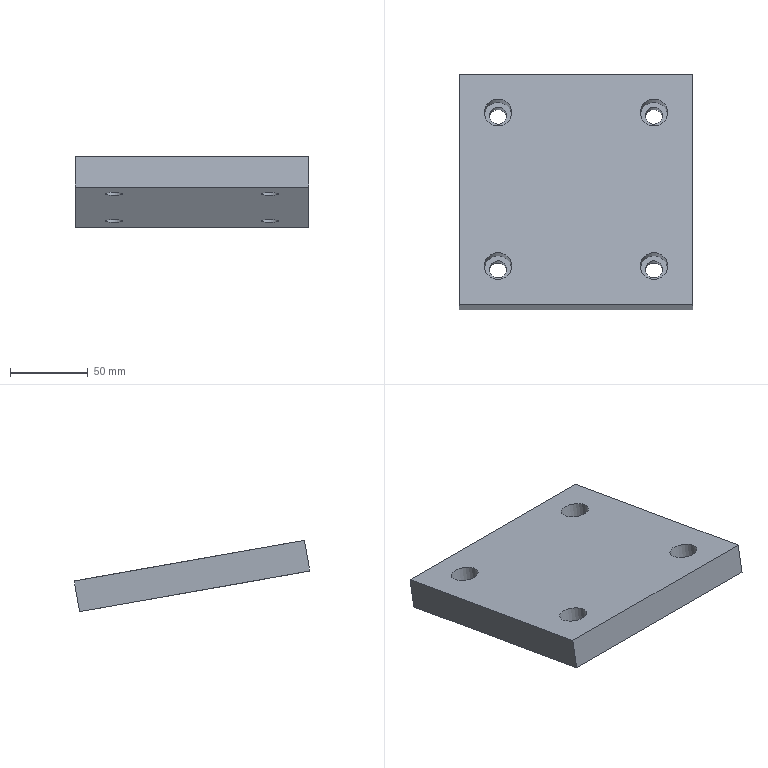Part | NX | features solid 2 | 1 solid | 18 faces | box 150 x 151.194 x 45.743 mm | volume 435414 mm3 | plane 10 | cylinder 8 | commonest cylinder face diameters 11 x4 17.5 x4
STEP:
#1=CARTESIAN_POINT('',(-801.6,-898.696,-239.036));
#2=VERTEX_POINT('',#1);
#3=CARTESIAN_POINT('',(-801.6,-902.169,-258.732));
#4=VERTEX_POINT('',#3);
#5=CARTESIAN_POINT('',(-801.6,-898.696,-239.036));
#6=DIRECTION('',(0.,0.1736,0.9848));
#7=VECTOR('',#6,1000.);
#8=LINE('',#5,#7);
#9=EDGE_CURVE('',#2,#4,#8,.F.);
#10=ORIENTED_EDGE('',*,*,#9,.T.);
#11=CARTESIAN_POINT('',(-951.6,-902.169,-258.732));
#12=VERTEX_POINT('',#11);
#13=CARTESIAN_POINT('',(-801.6,-902.169,-258.732));
#14=DIRECTION('',(1.,0.,0.));
#15=VECTOR('',#14,1000.);
#16=LINE('',#13,#15);
#17=EDGE_CURVE('',#4,#12,#16,.F.);
#18=ORIENTED_EDGE('',*,*,#17,.T.);
#19=CARTESIAN_POINT('',(-951.6,-898.696,-239.036));
#20=VERTEX_POINT('',#19);
#21=CARTESIAN_POINT('',(-951.6,-898.696,-239.036));
#22=DIRECTION('',(0.,-0.1736,-0.9848));
#23=VECTOR('',#22,1000.);
#24=LINE('',#21,#23);
#25=EDGE_CURVE('',#20,#12,#24,.T.);
#26=ORIENTED_EDGE('',*,*,#25,.F.);
#27=CARTESIAN_POINT('',(-801.6,-898.696,-239.036));
#28=DIRECTION('',(1.,0.,0.));
#29=VECTOR('',#28,1000.);
#30=LINE('',#27,#29);
#31=EDGE_CURVE('',#2,#20,#30,.F.);
#32=ORIENTED_EDGE('',*,*,#31,.F.);
#33=EDGE_LOOP('',(#10,#18,#26,#32));
#34=FACE_BOUND('',#33,.T.);
#35=CARTESIAN_POINT('',(-801.6,-898.696,-239.036));
#36=DIRECTION('',(0.,0.9848,-0.1736));
#37=DIRECTION('',(-1.,0.,0.));
#38=AXIS2_PLACEMENT_3D('',#35,#36,#37);
#39=PLANE('',#38);
#40=ADVANCED_FACE('',(#34),#39,.T.);
#41=ORIENTED_EDGE('',*,*,#25,.T.);
#42=CARTESIAN_POINT('',(-951.6,-1049.891,-232.685));
#43=VERTEX_POINT('',#42);
#44=CARTESIAN_POINT('',(-951.6,-852.929,-267.415));
#45=DIRECTION('',(0.,-0.9848,0.1736));
#46=VECTOR('',#45,1000.);
#47=LINE('',#44,#46);
#48=EDGE_CURVE('',#12,#43,#47,.T.);
#49=ORIENTED_EDGE('',*,*,#48,.T.);
#50=CARTESIAN_POINT('',(-951.6,-1046.418,-212.989));
#51=VERTEX_POINT('',#50);
#52=CARTESIAN_POINT('',(-951.6,-1046.418,-212.989));
#53=DIRECTION('',(0.,0.1736,0.9848));
#54=VECTOR('',#53,1000.);
#55=LINE('',#52,#54);
#56=EDGE_CURVE('',#51,#43,#55,.F.);
#57=ORIENTED_EDGE('',*,*,#56,.F.);
#58=CARTESIAN_POINT('',(-951.6,-849.456,-247.718));
#59=DIRECTION('',(0.,-0.9848,0.1736));
#60=VECTOR('',#59,1000.);
#61=LINE('',#58,#60);
#62=EDGE_CURVE('',#20,#51,#61,.T.);
#63=ORIENTED_EDGE('',*,*,#62,.F.);
#64=EDGE_LOOP('',(#41,#49,#57,#63));
#65=FACE_BOUND('',#64,.T.);
#66=CARTESIAN_POINT('',(-951.6,-849.456,-247.718));
#67=DIRECTION('',(-1.,0.,0.));
#68=DIRECTION('',(0.,-0.9848,0.1736));
#69=AXIS2_PLACEMENT_3D('',#66,#67,#68);
#70=PLANE('',#69);
#71=ADVANCED_FACE('',(#65),#70,.T.);
#72=ORIENTED_EDGE('',*,*,#56,.T.);
#73=CARTESIAN_POINT('',(-801.6,-1049.891,-232.685));
#74=VERTEX_POINT('',#73);
#75=CARTESIAN_POINT('',(-801.6,-1049.891,-232.685));
#76=DIRECTION('',(-1.,0.,0.));
#77=VECTOR('',#76,1000.);
#78=LINE('',#75,#77);
#79=EDGE_CURVE('',#74,#43,#78,.T.);
#80=ORIENTED_EDGE('',*,*,#79,.F.);
#81=CARTESIAN_POINT('',(-801.6,-1046.418,-212.989));
#82=VERTEX_POINT('',#81);
#83=CARTESIAN_POINT('',(-801.6,-1046.418,-212.989));
#84=DIRECTION('',(0.,0.1736,0.9848));
#85=VECTOR('',#84,1000.);
#86=LINE('',#83,#85);
#87=EDGE_CURVE('',#82,#74,#86,.F.);
#88=ORIENTED_EDGE('',*,*,#87,.F.);
#89=CARTESIAN_POINT('',(-801.6,-1046.418,-212.989));
#90=DIRECTION('',(-1.,0.,0.));
#91=VECTOR('',#90,1000.);
#92=LINE('',#89,#91);
#93=EDGE_CURVE('',#82,#51,#92,.T.);
#94=ORIENTED_EDGE('',*,*,#93,.T.);
#95=EDGE_LOOP('',(#72,#80,#88,#94));
#96=FACE_BOUND('',#95,.T.);
#97=CARTESIAN_POINT('',(-801.6,-1046.418,-212.989));
#98=DIRECTION('',(0.,0.9848,-0.1736));
#99=DIRECTION('',(-1.,0.,0.));
#100=AXIS2_PLACEMENT_3D('',#97,#98,#99);
#101=PLANE('',#100);
#102=ADVANCED_FACE('',(#96),#101,.F.);
#103=CARTESIAN_POINT('',(-801.6,-849.456,-247.718));
#104=DIRECTION('',(0.,-0.9848,0.1736));
#105=VECTOR('',#104,1000.);
#106=LINE('',#103,#105);
#107=EDGE_CURVE('',#2,#82,#106,.T.);
#108=ORIENTED_EDGE('',*,*,#107,.T.);
#109=ORIENTED_EDGE('',*,*,#87,.T.);
#110=CARTESIAN_POINT('',(-801.6,-852.929,-267.415));
#111=DIRECTION('',(0.,-0.9848,0.1736));
#112=VECTOR('',#111,1000.);
#113=LINE('',#110,#112);
#114=EDGE_CURVE('',#4,#74,#113,.T.);
#115=ORIENTED_EDGE('',*,*,#114,.F.);
#116=ORIENTED_EDGE('',*,*,#9,.F.);
#117=EDGE_LOOP('',(#108,#109,#115,#116));
#118=FACE_BOUND('',#117,.T.);
#119=CARTESIAN_POINT('',(-801.6,-849.456,-247.718));
#120=DIRECTION('',(-1.,0.,0.));
#121=DIRECTION('',(0.,-0.9848,0.1736));
#122=AXIS2_PLACEMENT_3D('',#119,#120,#121);
#123=PLANE('',#122);
#124=ADVANCED_FACE('',(#118),#123,.F.);
#125=CARTESIAN_POINT('',(-832.1,-926.79,-254.391));
#126=VERTEX_POINT('',#125);
#127=CARTESIAN_POINT('',(-826.6,-926.79,-254.391));
#128=DIRECTION('',(0.,0.1736,0.9848));
#129=DIRECTION('',(-1.,0.,0.));
#130=AXIS2_PLACEMENT_3D('',#127,#128,#129);
#131=CIRCLE('',#130,5.5);
#132=EDGE_CURVE('',#126,#126,#131,.T.);
#133=ORIENTED_EDGE('',*,*,#132,.T.);
#134=EDGE_LOOP('',(#133));
#135=FACE_BOUND('',#134,.T.);
#136=CARTESIAN_POINT('',(-932.1,-926.79,-254.391));
#137=VERTEX_POINT('',#136);
#138=CARTESIAN_POINT('',(-926.6,-926.79,-254.391));
#139=DIRECTION('',(0.,0.1736,0.9848));
#140=DIRECTION('',(-1.,0.,0.));
#141=AXIS2_PLACEMENT_3D('',#138,#139,#140);
#142=CIRCLE('',#141,5.5);
#143=EDGE_CURVE('',#137,#137,#142,.T.);
#144=ORIENTED_EDGE('',*,*,#143,.T.);
#145=EDGE_LOOP('',(#144));
#146=FACE_BOUND('',#145,.T.);
#147=CARTESIAN_POINT('',(-932.1,-1025.27,-237.026));
#148=VERTEX_POINT('',#147);
#149=CARTESIAN_POINT('',(-926.6,-1025.27,-237.026));
#150=DIRECTION('',(0.,0.1736,0.9848));
#151=DIRECTION('',(-1.,0.,0.));
#152=AXIS2_PLACEMENT_3D('',#149,#150,#151);
#153=CIRCLE('',#152,5.5);
#154=EDGE_CURVE('',#148,#148,#153,.T.);
#155=ORIENTED_EDGE('',*,*,#154,.T.);
#156=EDGE_LOOP('',(#155));
#157=FACE_BOUND('',#156,.T.);
#158=CARTESIAN_POINT('',(-832.1,-1025.27,-237.026));
#159=VERTEX_POINT('',#158);
#160=CARTESIAN_POINT('',(-826.6,-1025.27,-237.026));
#161=DIRECTION('',(0.,0.1736,0.9848));
#162=DIRECTION('',(-1.,0.,0.));
#163=AXIS2_PLACEMENT_3D('',#160,#161,#162);
#164=CIRCLE('',#163,5.5);
#165=EDGE_CURVE('',#159,#159,#164,.T.);
#166=ORIENTED_EDGE('',*,*,#165,.T.);
#167=EDGE_LOOP('',(#166));
#168=FACE_BOUND('',#167,.T.);
#169=ORIENTED_EDGE('',*,*,#79,.T.);
#170=ORIENTED_EDGE('',*,*,#48,.F.);
#171=ORIENTED_EDGE('',*,*,#17,.F.);
#172=ORIENTED_EDGE('',*,*,#114,.T.);
#173=EDGE_LOOP('',(#169,#170,#171,#172));
#174=FACE_BOUND('',#173,.T.);
#175=CARTESIAN_POINT('',(-801.6,-852.929,-267.415));
#176=DIRECTION('',(0.,0.1736,0.9848));
#177=DIRECTION('',(-1.,0.,0.));
#178=AXIS2_PLACEMENT_3D('',#175,#176,#177);
#179=PLANE('',#178);
#180=ADVANCED_FACE('',(#135,#146,#157,#168,#174),#179,.F.);
#181=CARTESIAN_POINT('',(-817.85,-923.317,-234.695));
#182=VERTEX_POINT('',#181);
#183=CARTESIAN_POINT('',(-826.6,-923.317,-234.695));
#184=DIRECTION('',(0.,-0.1736,-0.9848));
#185=DIRECTION('',(1.,0.,0.));
#186=AXIS2_PLACEMENT_3D('',#183,#184,#185);
#187=CIRCLE('',#186,8.75);
#188=EDGE_CURVE('',#182,#182,#187,.T.);
#189=ORIENTED_EDGE('',*,*,#188,.T.);
#190=EDGE_LOOP('',(#189));
#191=FACE_BOUND('',#190,.T.);
#192=CARTESIAN_POINT('',(-917.85,-923.317,-234.695));
#193=VERTEX_POINT('',#192);
#194=CARTESIAN_POINT('',(-926.6,-923.317,-234.695));
#195=DIRECTION('',(0.,-0.1736,-0.9848));
#196=DIRECTION('',(1.,0.,0.));
#197=AXIS2_PLACEMENT_3D('',#194,#195,#196);
#198=CIRCLE('',#197,8.75);
#199=EDGE_CURVE('',#193,#193,#198,.T.);
#200=ORIENTED_EDGE('',*,*,#199,.T.);
#201=EDGE_LOOP('',(#200));
#202=FACE_BOUND('',#201,.T.);
#203=CARTESIAN_POINT('',(-917.85,-1021.797,-217.33));
#204=VERTEX_POINT('',#203);
#205=CARTESIAN_POINT('',(-926.6,-1021.797,-217.33));
#206=DIRECTION('',(0.,-0.1736,-0.9848));
#207=DIRECTION('',(1.,0.,0.));
#208=AXIS2_PLACEMENT_3D('',#205,#206,#207);
#209=CIRCLE('',#208,8.75);
#210=EDGE_CURVE('',#204,#204,#209,.T.);
#211=ORIENTED_EDGE('',*,*,#210,.T.);
#212=EDGE_LOOP('',(#211));
#213=FACE_BOUND('',#212,.T.);
#214=CARTESIAN_POINT('',(-817.85,-1021.797,-217.33));
#215=VERTEX_POINT('',#214);
#216=CARTESIAN_POINT('',(-826.6,-1021.797,-217.33));
#217=DIRECTION('',(0.,-0.1736,-0.9848));
#218=DIRECTION('',(1.,0.,0.));
#219=AXIS2_PLACEMENT_3D('',#216,#217,#218);
#220=CIRCLE('',#219,8.75);
#221=EDGE_CURVE('',#215,#215,#220,.T.);
#222=ORIENTED_EDGE('',*,*,#221,.T.);
#223=EDGE_LOOP('',(#222));
#224=FACE_BOUND('',#223,.T.);
#225=ORIENTED_EDGE('',*,*,#93,.F.);
#226=ORIENTED_EDGE('',*,*,#107,.F.);
#227=ORIENTED_EDGE('',*,*,#31,.T.);
#228=ORIENTED_EDGE('',*,*,#62,.T.);
#229=EDGE_LOOP('',(#225,#226,#227,#228));
#230=FACE_BOUND('',#229,.T.);
#231=CARTESIAN_POINT('',(-801.6,-849.456,-247.718));
#232=DIRECTION('',(0.,0.1736,0.9848));
#233=DIRECTION('',(-1.,0.,0.));
#234=AXIS2_PLACEMENT_3D('',#231,#232,#233);
#235=PLANE('',#234);
#236=ADVANCED_FACE('',(#191,#202,#213,#224,#230),#235,.T.);
#237=CARTESIAN_POINT('',(-821.1,-1023.881,-229.148));
#238=VERTEX_POINT('',#237);
#239=CARTESIAN_POINT('',(-826.6,-1023.881,-229.148));
#240=DIRECTION('',(0.,-0.1736,-0.9848));
#241=DIRECTION('',(1.,0.,0.));
#242=AXIS2_PLACEMENT_3D('',#239,#240,#241);
#243=CIRCLE('',#242,5.5);
#244=EDGE_CURVE('',#238,#238,#243,.T.);
#245=ORIENTED_EDGE('',*,*,#244,.F.);
#246=EDGE_LOOP('',(#245));
#247=FACE_BOUND('',#246,.T.);
#248=ORIENTED_EDGE('',*,*,#165,.F.);
#249=EDGE_LOOP('',(#248));
#250=FACE_BOUND('',#249,.T.);
#251=CARTESIAN_POINT('',(-826.6,-1030.48,-266.57));
#252=DIRECTION('',(0.,-0.1736,-0.9848));
#253=DIRECTION('',(1.,0.,0.));
#254=AXIS2_PLACEMENT_3D('',#251,#252,#253);
#255=CYLINDRICAL_SURFACE('',#254,5.5);
#256=ADVANCED_FACE('',(#247,#250),#255,.F.);
#257=ORIENTED_EDGE('',*,*,#244,.T.);
#258=EDGE_LOOP('',(#257));
#259=FACE_BOUND('',#258,.T.);
#260=CARTESIAN_POINT('',(-817.85,-1023.881,-229.148));
#261=VERTEX_POINT('',#260);
#262=CARTESIAN_POINT('',(-826.6,-1023.881,-229.148));
#263=DIRECTION('',(0.,-0.1736,-0.9848));
#264=DIRECTION('',(1.,0.,0.));
#265=AXIS2_PLACEMENT_3D('',#262,#263,#264);
#266=CIRCLE('',#265,8.75);
#267=EDGE_CURVE('',#261,#261,#266,.T.);
#268=ORIENTED_EDGE('',*,*,#267,.F.);
#269=EDGE_LOOP('',(#268));
#270=FACE_BOUND('',#269,.T.);
#271=CARTESIAN_POINT('',(-826.6,-1023.881,-229.148));
#272=DIRECTION('',(0.,-0.1736,-0.9848));
#273=DIRECTION('',(1.,0.,0.));
#274=AXIS2_PLACEMENT_3D('',#271,#272,#273);
#275=PLANE('',#274);
#276=ADVANCED_FACE('',(#259,#270),#275,.F.);
#277=ORIENTED_EDGE('',*,*,#267,.T.);
#278=EDGE_LOOP('',(#277));
#279=FACE_BOUND('',#278,.T.);
#280=ORIENTED_EDGE('',*,*,#221,.F.);
#281=EDGE_LOOP('',(#280));
#282=FACE_BOUND('',#281,.T.);
#283=CARTESIAN_POINT('',(-826.6,-1021.797,-217.33));
#284=DIRECTION('',(0.,-0.1736,-0.9848));
#285=DIRECTION('',(1.,0.,0.));
#286=AXIS2_PLACEMENT_3D('',#283,#284,#285);
#287=CYLINDRICAL_SURFACE('',#286,8.75);
#288=ADVANCED_FACE('',(#279,#282),#287,.F.);
#289=CARTESIAN_POINT('',(-921.1,-1023.881,-229.148));
#290=VERTEX_POINT('',#289);
#291=CARTESIAN_POINT('',(-926.6,-1023.881,-229.148));
#292=DIRECTION('',(0.,-0.1736,-0.9848));
#293=DIRECTION('',(1.,0.,0.));
#294=AXIS2_PLACEMENT_3D('',#291,#292,#293);
#295=CIRCLE('',#294,5.5);
#296=EDGE_CURVE('',#290,#290,#295,.T.);
#297=ORIENTED_EDGE('',*,*,#296,.F.);
#298=EDGE_LOOP('',(#297));
#299=FACE_BOUND('',#298,.T.);
#300=ORIENTED_EDGE('',*,*,#154,.F.);
#301=EDGE_LOOP('',(#300));
#302=FACE_BOUND('',#301,.T.);
#303=CARTESIAN_POINT('',(-926.6,-1030.48,-266.57));
#304=DIRECTION('',(0.,-0.1736,-0.9848));
#305=DIRECTION('',(1.,0.,0.));
#306=AXIS2_PLACEMENT_3D('',#303,#304,#305);
#307=CYLINDRICAL_SURFACE('',#306,5.5);
#308=ADVANCED_FACE('',(#299,#302),#307,.F.);
#309=ORIENTED_EDGE('',*,*,#296,.T.);
#310=EDGE_LOOP('',(#309));
#311=FACE_BOUND('',#310,.T.);
#312=CARTESIAN_POINT('',(-917.85,-1023.881,-229.148));
#313=VERTEX_POINT('',#312);
#314=CARTESIAN_POINT('',(-926.6,-1023.881,-229.148));
#315=DIRECTION('',(0.,-0.1736,-0.9848));
#316=DIRECTION('',(1.,0.,0.));
#317=AXIS2_PLACEMENT_3D('',#314,#315,#316);
#318=CIRCLE('',#317,8.75);
#319=EDGE_CURVE('',#313,#313,#318,.T.);
#320=ORIENTED_EDGE('',*,*,#319,.F.);
#321=EDGE_LOOP('',(#320));
#322=FACE_BOUND('',#321,.T.);
#323=CARTESIAN_POINT('',(-926.6,-1023.881,-229.148));
#324=DIRECTION('',(0.,-0.1736,-0.9848));
#325=DIRECTION('',(1.,0.,0.));
#326=AXIS2_PLACEMENT_3D('',#323,#324,#325);
#327=PLANE('',#326);
#328=ADVANCED_FACE('',(#311,#322),#327,.F.);
#329=ORIENTED_EDGE('',*,*,#319,.T.);
#330=EDGE_LOOP('',(#329));
#331=FACE_BOUND('',#330,.T.);
#332=ORIENTED_EDGE('',*,*,#210,.F.);
#333=EDGE_LOOP('',(#332));
#334=FACE_BOUND('',#333,.T.);
#335=CARTESIAN_POINT('',(-926.6,-1021.797,-217.33));
#336=DIRECTION('',(0.,-0.1736,-0.9848));
#337=DIRECTION('',(1.,0.,0.));
#338=AXIS2_PLACEMENT_3D('',#335,#336,#337);
#339=CYLINDRICAL_SURFACE('',#338,8.75);
#340=ADVANCED_FACE('',(#331,#334),#339,.F.);
#341=CARTESIAN_POINT('',(-921.1,-925.4,-246.513));
#342=VERTEX_POINT('',#341);
#343=CARTESIAN_POINT('',(-926.6,-925.4,-246.513));
#344=DIRECTION('',(0.,-0.1736,-0.9848));
#345=DIRECTION('',(1.,0.,0.));
#346=AXIS2_PLACEMENT_3D('',#343,#344,#345);
#347=CIRCLE('',#346,5.5);
#348=EDGE_CURVE('',#342,#342,#347,.T.);
#349=ORIENTED_EDGE('',*,*,#348,.F.);
#350=EDGE_LOOP('',(#349));
#351=FACE_BOUND('',#350,.T.);
#352=ORIENTED_EDGE('',*,*,#143,.F.);
#353=EDGE_LOOP('',(#352));
#354=FACE_BOUND('',#353,.T.);
#355=CARTESIAN_POINT('',(-926.6,-931.999,-283.935));
#356=DIRECTION('',(0.,-0.1736,-0.9848));
#357=DIRECTION('',(1.,0.,0.));
#358=AXIS2_PLACEMENT_3D('',#355,#356,#357);
#359=CYLINDRICAL_SURFACE('',#358,5.5);
#360=ADVANCED_FACE('',(#351,#354),#359,.F.);
#361=ORIENTED_EDGE('',*,*,#348,.T.);
#362=EDGE_LOOP('',(#361));
#363=FACE_BOUND('',#362,.T.);
#364=CARTESIAN_POINT('',(-917.85,-925.4,-246.513));
#365=VERTEX_POINT('',#364);
#366=CARTESIAN_POINT('',(-926.6,-925.4,-246.513));
#367=DIRECTION('',(0.,-0.1736,-0.9848));
#368=DIRECTION('',(1.,0.,0.));
#369=AXIS2_PLACEMENT_3D('',#366,#367,#368);
#370=CIRCLE('',#369,8.75);
#371=EDGE_CURVE('',#365,#365,#370,.T.);
#372=ORIENTED_EDGE('',*,*,#371,.F.);
#373=EDGE_LOOP('',(#372));
#374=FACE_BOUND('',#373,.T.);
#375=CARTESIAN_POINT('',(-926.6,-925.4,-246.513));
#376=DIRECTION('',(0.,-0.1736,-0.9848));
#377=DIRECTION('',(1.,0.,0.));
#378=AXIS2_PLACEMENT_3D('',#375,#376,#377);
#379=PLANE('',#378);
#380=ADVANCED_FACE('',(#363,#374),#379,.F.);
#381=ORIENTED_EDGE('',*,*,#371,.T.);
#382=EDGE_LOOP('',(#381));
#383=FACE_BOUND('',#382,.T.);
#384=ORIENTED_EDGE('',*,*,#199,.F.);
#385=EDGE_LOOP('',(#384));
#386=FACE_BOUND('',#385,.T.);
#387=CARTESIAN_POINT('',(-926.6,-923.317,-234.695));
#388=DIRECTION('',(0.,-0.1736,-0.9848));
#389=DIRECTION('',(1.,0.,0.));
#390=AXIS2_PLACEMENT_3D('',#387,#388,#389);
#391=CYLINDRICAL_SURFACE('',#390,8.75);
#392=ADVANCED_FACE('',(#383,#386),#391,.F.);
#393=CARTESIAN_POINT('',(-821.1,-925.4,-246.513));
#394=VERTEX_POINT('',#393);
#395=CARTESIAN_POINT('',(-826.6,-925.4,-246.513));
#396=DIRECTION('',(0.,-0.1736,-0.9848));
#397=DIRECTION('',(1.,0.,0.));
#398=AXIS2_PLACEMENT_3D('',#395,#396,#397);
#399=CIRCLE('',#398,5.5);
#400=EDGE_CURVE('',#394,#394,#399,.T.);
#401=ORIENTED_EDGE('',*,*,#400,.F.);
#402=EDGE_LOOP('',(#401));
#403=FACE_BOUND('',#402,.T.);
#404=ORIENTED_EDGE('',*,*,#132,.F.);
#405=EDGE_LOOP('',(#404));
#406=FACE_BOUND('',#405,.T.);
#407=CARTESIAN_POINT('',(-826.6,-931.999,-283.935));
#408=DIRECTION('',(0.,-0.1736,-0.9848));
#409=DIRECTION('',(1.,0.,0.));
#410=AXIS2_PLACEMENT_3D('',#407,#408,#409);
#411=CYLINDRICAL_SURFACE('',#410,5.5);
#412=ADVANCED_FACE('',(#403,#406),#411,.F.);
#413=ORIENTED_EDGE('',*,*,#400,.T.);
#414=EDGE_LOOP('',(#413));
#415=FACE_BOUND('',#414,.T.);
#416=CARTESIAN_POINT('',(-817.85,-925.4,-246.513));
#417=VERTEX_POINT('',#416);
#418=CARTESIAN_POINT('',(-826.6,-925.4,-246.513));
#419=DIRECTION('',(0.,-0.1736,-0.9848));
#420=DIRECTION('',(1.,0.,0.));
#421=AXIS2_PLACEMENT_3D('',#418,#419,#420);
#422=CIRCLE('',#421,8.75);
#423=EDGE_CURVE('',#417,#417,#422,.T.);
#424=ORIENTED_EDGE('',*,*,#423,.F.);
#425=EDGE_LOOP('',(#424));
#426=FACE_BOUND('',#425,.T.);
#427=CARTESIAN_POINT('',(-826.6,-925.4,-246.513));
#428=DIRECTION('',(0.,-0.1736,-0.9848));
#429=DIRECTION('',(1.,0.,0.));
#430=AXIS2_PLACEMENT_3D('',#427,#428,#429);
#431=PLANE('',#430);
#432=ADVANCED_FACE('',(#415,#426),#431,.F.);
#433=ORIENTED_EDGE('',*,*,#423,.T.);
#434=EDGE_LOOP('',(#433));
#435=FACE_BOUND('',#434,.T.);
#436=ORIENTED_EDGE('',*,*,#188,.F.);
#437=EDGE_LOOP('',(#436));
#438=FACE_BOUND('',#437,.T.);
#439=CARTESIAN_POINT('',(-826.6,-923.317,-234.695));
#440=DIRECTION('',(0.,-0.1736,-0.9848));
#441=DIRECTION('',(1.,0.,0.));
#442=AXIS2_PLACEMENT_3D('',#439,#440,#441);
#443=CYLINDRICAL_SURFACE('',#442,8.75);
#444=ADVANCED_FACE('',(#435,#438),#443,.F.);
#445=CLOSED_SHELL('',(#40,#71,#102,#124,#180,#236,#256,#276,#288,#308,#328,#340,#360,#380,#392,#412,#432,#444));
#446=MANIFOLD_SOLID_BREP('',#445);
#447=(LENGTH_UNIT()NAMED_UNIT(*)SI_UNIT(.MILLI.,.METRE.));
#448=UNCERTAINTY_MEASURE_WITH_UNIT(LENGTH_MEASURE(0.00001),#447,'','');
#449=(NAMED_UNIT(*)PLANE_ANGLE_UNIT()SI_UNIT($,.RADIAN.));
#450=(NAMED_UNIT(*)SI_UNIT($,.STERADIAN.)SOLID_ANGLE_UNIT());
#451=(GEOMETRIC_REPRESENTATION_CONTEXT(3)GLOBAL_UNCERTAINTY_ASSIGNED_CONTEXT((#448))GLOBAL_UNIT_ASSIGNED_CONTEXT((#447,#449,#450))REPRESENTATION_CONTEXT('',''));
#452=ADVANCED_BREP_SHAPE_REPRESENTATION('',(#446),#451);